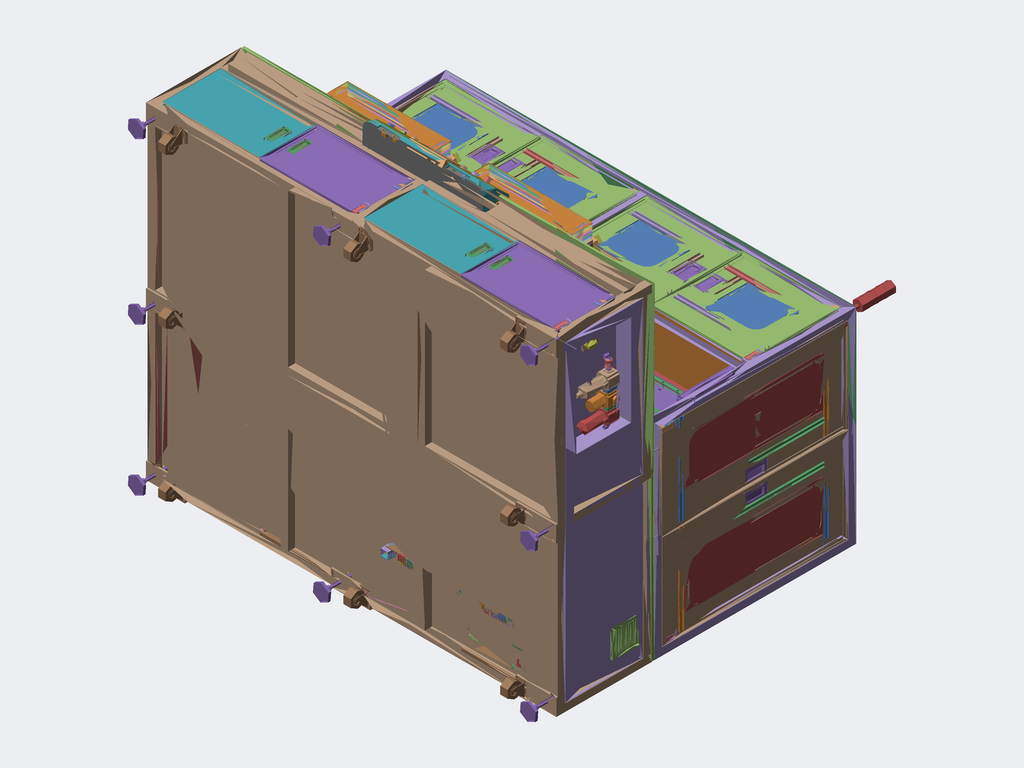Assembly | STEP file | 226 different items | 645 placed
Parts list (item | name | quantity | parent item | size | volume):
1 | ball screw nut-SFA3232-2.8 | x1 | - | 62 x 80 x 110 mm | 157675 mm3
2 | - | x1 | - | 31 x 2020 x 31 mm | 1487693 mm3
3 | HIWIN linear rail EGH30-1920-40-40 | x2 | in HIWIN linear rail EGH30CA | 28 x 23 x 1920 mm | 1071300 mm3
4 | HIWIN slider EGH30CA | x4 | in HIWIN linear rail EGH30CA | 60 x 32 x 99.1 mm | 151904 mm3
5 | - | x1 | - | 1970 x 20 x 225 mm | 8481911 mm3
6 | - | x1 | - | 11.5 x 66 x 40 mm | 3360 mm3
7 | - | x1 | - | 217 x 63 x 320 mm | 1789943 mm3
8 | - | x1 | - | 105 x 159 x 12 mm | 123349 mm3
9 | - | x1 | - | 319 x 74 x 2 mm | 46848 mm3
10 | - | x1 | - | 319 x 74 x 2 mm | 41628 mm3
11 | - | x1 | - | 100 x 108 x 18.001 mm | 56664 mm3
12 | - | x1 | - | 40 x 10 x 30 mm | 9955 mm3
13 | - | x1 | - | 110 x 160 x 60 mm | 79904 mm3
14 | - | x4 | - | 58 x 58 x 14 mm | 28098 mm3
15 | - | x1 | - | 152 x 125 x 238 mm | 147473 mm3
16 | - | x1 | - | 180 x 125 x 238 mm | 188317 mm3
17 | - | x2 | - | 230 x 2 x 105 mm | 25066 mm3
18 | - | x2 | - | - | -
19 | timing pulley C-HTPA30S5M250-A-N19 | x1 | - | 32 x 52 x 52 mm | 41096 mm3
20 | timing pulley C-HTPA30S5M250-A-N20 | x1 | - | 32 x 52 x 52 mm | 40136 mm3
21 | slot-type photoelectric sensor LU672-5N | x1 | - | 14.05 x 26.2 x 61.3 mm | 1669 mm3
22 | bearing fixing block BF25 | x1 | - | 30 x 106 x 80 mm | 180921 mm3
23 | bearing support block BK25 | x1 | - | 106 x 63 x 80 mm | 295057 mm3
24 | GB/T 894-2017 external retaining ring type A 25 | x1 | - | 27.3 x 30.557 x 1.2 mm | 213.948 mm3
25 | Heqi servo 1000W motor X2MA100A-N2L (aviation plug) | x1 | - | - | -
26 | - | x1 | - | 183.34 x 51.65 x 25 mm | 35272 mm3
27 | ball screw nut-SFS02525-1.8 | x2 | - | 48 x 62 x 60 mm | 60127 mm3
28 | - | x2 | - | 25 x 970 x 25 mm | 453168 mm3
29 | slider HGW30HC | x8 | - | 90 x 36 x 120.7 mm | 241575 mm3
30 | linear guide HGR30HC-1250-25-25 | x4 | - | 28 x 26 x 1250 mm | 722759 mm3
31 | - | x2 | in 211 | 570 x 570 x 15 mm | 4074607 mm3
32 | - | x2 | in 211 | 61.9 x 61.9 x 60 mm | 168821 mm3
33 | - | x4 | in 211 | 88 x 56 x 10 mm | 42549 mm3
34 | - | x2 | in 211 | 6.3 x 100 x 6.3 mm | 3083 mm3
35 | - | x2 | in 211 | 59.5 x 40 x 25 mm | 15043 mm3
36 | - | x4 | in 211 | 130 x 35 x 30 mm | 74604 mm3
37 | - | x4 | in 211 | 60 x 35 x 10 mm | 20336 mm3
38 | rotary cylinder ACKL32x90 | x4 | in 211 | 54 x 76 x 54 mm | 144312 mm3
39 | - | x2 | in 211 | 360 x 72.5 x 360 mm | 3129469 mm3
40 | - | x2 | in 211 | 419 x 78.97 x 419 mm | 4583187 mm3
41 | - | x2 | in 211 | 452 x 75.25 x 452 mm | 5130306 mm3
42 | - | x2 | in 211 | 520 x 79.32 x 520 mm | 7165293 mm3
43 | - | x4 | in Y-axis bellows cover assembly | 570 x 2 x 115 mm | 37091 mm3
44 | - | x4 | in Y-axis bellows cover assembly | 570 x 35 x 115.5 mm | 243087 mm3
45 | - | x4 | in Y-axis bellows cover assembly | - | -
46 | - | x2 | - | 80 x 85 x 125 mm | 372147 mm3
47 | - | x2 | - | 75 x 75 x 15 mm | 51651 mm3
48 | - | x2 | - | 65 x 82.5 x 45 mm | 171264 mm3
49 | - | x8 | - | 95 x 63 x 75 mm | 244424 mm3
50 | - | x2 | - | 13.5 x 37 x 40 mm | 2353 mm3
51 | - | x2 | - | 80 x 1.2 x 95 mm | 9034 mm3
52 | - | x4 | - | 35 x 20 x 30 mm | 2265 mm3
53 | - | x4 | - | 570 x 114 x 2 mm | 119896 mm3
54 | anti-collision silicone pad | x2 | - | 34 x 10 x 7 mm | 2064 mm3
55 | coupling DEP12-D40L-d17-e19-DC-DD | x2 | - | 66 x 40 x 41.384 mm | 61965 mm3
56 | GB/T 276-2013 deep groove ball bearing 6004-2RZ_6004-2RZ | x2 | - | 12 x 42 x 42 mm | 9713 mm3
57 | GB/T 894-2017[external retaining ring type A 20MM_20 | x2 | - | 22.1 x 25.046 x 1.2 mm | 154.505 mm3
58 | TBI bearing block FK20 | x2 | - | 85 x 85 x 64 mm | 139023 mm3
59 | Heqi 750W servo (SV-2MH075A-N2-LN wire type) | x2 | - | - | -
60 | slot-type photoelectric LU674-5NA | x2 | - | 15 x 16 x 28 mm | 2937 mm3
61 | - | x2 | - | 533 x 321 x 16 mm | 246500 mm3
62 | mirrored door latch (COMPANY_B) | x20 | in 68, 122, 127, 129 | 93 x 9.976 x 34.988 mm | 6427 mm3
63 | door latch (COMPANY_B) | x20 | in 68, 122, 127, 129 | 93 x 9.976 x 34.988 mm | 6427 mm3
64 | GY-AA29-AL06-96 nylon handle | x8 | in 68 | 43 x 107 x 15 mm | 16385 mm3
65 | door handle rear cover (SUS304) | x8 | in 68 | 47 x 108 x 11 mm | 7052 mm3
66 | - | x2 | in 68 | 533 x 321 x 15 mm | 244434 mm3
67 | - | x2 | - | 533 x 428 x 16 mm | 320755 mm3
68 | - | x2 | in 68 | 533 x 428 x 15 mm | 318433 mm3
69 | - | x1 | in 69 | 660.4 x 129.2 x 145.9 mm | 256487 mm3
70 | HMI touch panel SK-070QE.V1.5 | x1 | in 69 | 203 x 145 x 39 mm | 1003292 mm3
71 | three-pin two-speed power switch KCD4-16A-250 | x1 | in 69 | 21 x 15 x 27.336 mm | 4367 mm3
72 | illuminated flat push button white 24V | x1 | in 69 | 30 x 38 x 66.5 mm | 57717 mm3
73 | Yijia emergency stop switch | x1 | in 69 | 83 x 36 x 36 mm | 62929 mm3
74 | illuminated flat push button yellow 24V | x1 | in 69 | 30 x 38 x 66.5 mm | 57717 mm3
75 | illuminated flat push button green 24V | x2 | in 69 | 30 x 38 x 66.5 mm | 57717 mm3
76 | illuminated flat push button red 24V | x1 | in 69 | 30 x 38 x 66.5 mm | 57717 mm3
77 | USB interface | x2 | in 69 | 38 x 27 x 12 mm | 7027 mm3
78 | handheld controller connector DB9-RS232 | x1 | in 69 | 32 x 27 x 13 mm | 4868 mm3
79 | - | x1 | in 214 | 870 x 460 x 3 mm | 1176521 mm3
80 | power supply fixing sheet metal | x2 | in 214 | 15 x 20 x 10 mm | 522.847 mm3
81 | terminal stopper UK2.5B | x1 | in relay slot group | 43 x 36 x 10 mm | 8109 mm3
82 | terminal block UK2.5B | x30 | in relay slot group | 43 x 41 x 6 mm | 4189 mm3
83 | IDEC relay RJ1S-A220 | x3 | in relay slot group | 71 x 56 x 15 mm | 30075 mm3
84 | card slot 35-265 | x1 | in relay slot group | 35 x 6.5 x 265 mm | 13977 mm3
85 | - | x4 | in 214 | 40 x 38.5 x 480 mm | 109641 mm3
86 | Mean Well power supply LRS-350-24 | x1 | in 214 | - | -
87 | filter CW4EL2-30A-S | x1 | in 214 | 85 x 51 x 29 mm | 93702 mm3
88 | contactor NXC-12 | x1 | in 214 | 75 x 85 x 45 mm | 200816 mm3
89 | circuit breaker DZ267LE-32-10 | x1 | in 214 | 75.5 x 84 x 36 mm | 154947 mm3
90 | - | x3 | in 214 | 40 x 38.5 x 320 mm | 73088 mm3
91 | - | x1 | in 214 | 316 x 26 x 94 mm | 418687 mm3
92 | Puge 400W electric screwdriver driver | x3 | in 214 | - | -
93 | Heqi 750W servo driver (X3EA075A-A2) | x2 | in 214 | - | -
94 | Heqi 1000W servo driver SV-X3EA100A-A2 | x1 | in 214 | - | -
95 | - | x1 | in 168 | 2260 x 16 x 1812 mm | 64799622 mm3
96 | - | x1 | in 168 | 1718 x 428 x 15 mm | 1162465 mm3
97 | - | x1 | in 168 | 1718 x 428 x 87.5 mm | 1351126 mm3
98 | - | x1 | in 168 | 2260 x 525 x 1800 mm | 63757591 mm3
99 | - | x3 | in 168 | 30 x 67 x 20 mm | 5371 mm3
100 | - | x2 | in 168 | 38 x 142 x 10 mm | 51461 mm3
101 | - | x1 | in 168 | 71.5 x 31.5 x 125 mm | 22831 mm3
102 | silencer fixing block | x1 | in 168 | 60 x 25 x 20 mm | 24053 mm3
103 | large foot pad | x8 | in 168 | 96 x 166 x 96 mm | 161391 mm3
104 | universal caster-cf | x8 | in 168 | 115.75 x 105.5 x 64.5 mm | 273240 mm3
105 | power switch 2 | x1 | in 168 | 64.5 x 99 x 64.5 mm | 195044 mm3
106 | upright fitting KQ2H08-02AS | x2 | in 168 | 16.166 x 22 x 14 mm | 2374 mm3
107 | louvered fan grille LA751PBX0307 | x2 | in 168 | 151 x 151 x 33 mm | 559203 mm3
108 | 220V fan | x2 | in 168 | - | -
109 | hand slide valve HSV10 | x1 | in 110 | 35.5 x 35.5 x 68.5 mm | 34566 mm3
110 | pneumatic FRL unit GAC40010AS | x1 | in 110 | 248 x 227 x 99 mm | 1724530 mm3
111 | L-type fitting PL1003 | x2 | in 110 | 35.315 x 37 x 18 mm | 6710 mm3
112 | 1-branch plug | x2 | in four-station solenoid valve block-double head | 9.5 x 8 x 9.5 mm | 424.158 mm3
113 | 2-branch plug | x3 | in four-station solenoid valve block-double head | 13 x 9 x 13 mm | 992.021 mm3
114 | L-type fitting PL4-01 | x4 | in four-station solenoid valve block-double head | 22.874 x 22.3 x 11 mm | 1653 mm3
115 | L-type fitting PL6-01 | x1 | in four-station solenoid valve block-double head | 23.774 x 24.5 x 13 mm | 2165 mm3
116 | L-type fitting PL8-01 | x1 | in four-station solenoid valve block-double head | 29.374 x 27.1 x 15 mm | 3387 mm3
117 | single solenoid valve MVSD-180-4E1 | x2 | in four-station solenoid valve block-double head | 33.5 x 18 x 107 mm | 44857 mm3
118 | double solenoid valve 4V120-06 | x2 | in four-station solenoid valve block-double head | 33.5 x 18 x 144.5 mm | 59015 mm3
119 | - | x1 | in four-station solenoid valve block-double head | 95 x 25 x 58 mm | 76550 mm3
120 | upright fitting APC8-02 | x3 | in four-station solenoid valve block-double head | 25.7 x 16.166 x 15 mm | 2429 mm3
121 | - | x1 | in 168 | 2260 x 1110 x 1130 mm | 31144835 mm3
122 | - | x4 | in 122 | 523 x 1028 x 15 mm | 879625 mm3
123 | - | x4 | in 122 | 274 x 764 x 5 mm | 1044923 mm3
124 | door handle XAC81_A128 | x12 | in 122, 127, 129 | 128 x 19.001 x 83 mm | 21652 mm3
125 | magnetic latch HGE11-52-L150 | x12 | in 122, 127, 129 | 60 x 15 x 37 mm | 14160 mm3
126 | magnetic door catch | x8 | in 122, 127 | 53 x 13 x 25.5 mm | 11239 mm3
127 | - | x4 | in 127 | 533 x 1028 x 15 mm | 886970 mm3
128 | - | x4 | in 127 | 284 x 764 x 5 mm | 1083123 mm3
129 | - | x4 | in 129 | 533 x 508 x 15 mm | 546675 mm3
130 | - | x4 | in 129 | 284 x 244 x 5 mm | 344723 mm3
131 | - | x1 | in 168 | 1130 x 2260 x 2 mm | 5103955 mm3
132 | foldable alarm light | x1 | in 168 | 70 x 342 x 70 mm | 623933 mm3
133 | STD-NB1220 safety light curtain | x4 | in 168 | 29 x 296.5 x 27 mm | 192265 mm3
134 | LED 0.9M T8 tube, single-end input 30W ZKT8-9-A-12 | x2 | in 168 | - | -
135 | - | x1 | - | 1500 x 280 x 500 mm | 11121240 mm3
136 | - | x1 | - | 500 x 1500 x 10 mm | 7485180 mm3
137 | COMPANY_C blow-air scheme, large part | x1 | - | 475 x 570.585 x 525.846 mm | 39693153 mm3
138 | COMPANY_C blow-air scheme, small part | x2 | - | 330.519 x 479.611 x 400.249 mm | 15256287 mm3
139 | - | x3 | - | 45 x 20 x 13 mm | 10795 mm3
140 | - | x3 | - | 50 x 24 x 8 mm | 8483 mm3
141 | - | x1 | - | 12 x 37 x 18 mm | 4359 mm3
142 | - | x1 | - | 12 x 37 x 18 mm | 4359 mm3
143 | - | x6 | - | 8 x 23.5 x 5 mm | 825.463 mm3
144 | finger cylinder MHZL2-16D | x3 | - | 47 x 23.6 x 70 mm | 34913 mm3
145 | speed control fitting AS1201F-M5-04SA | x6 | - | 9.4 x 26.5 x 22 mm | 1970 mm3
146 | through-beam fiber sensor FT-D321Q-M | x6 | - | 3 x 3 x 21 mm | 128.837 mm3
147 | - | x2 | - | 17.3 x 24.5 x 17.3 mm | 2659 mm3
148 | - | x2 | - | 12 x 30 x 18 mm | 3302 mm3
149 | - | x2 | - | 12 x 30 x 18 mm | 3302 mm3
150 | - | x3 | - | 9.9 x 14.5 x 9.9 mm | 641.755 mm3
151 | - | x3 | - | 9.9 x 15.5 x 9.9 mm | 641.291 mm3
152 | - | x1 | - | 350 x 190 x 10 mm | 648871 mm3
153 | - | x1 | - | 180 x 12 x 70 mm | 130133 mm3
154 | - | x1 | - | 45 x 27.5 x 10 mm | 9795 mm3
155 | - | x1 | - | 30 x 40 x 18 mm | 14417 mm3
156 | - | x1 | - | 350 x 150 x 10 mm | 449712 mm3
157 | - | x6 | - | 20 x 20 x 110 mm | 33959 mm3
158 | - | x1 | - | 65 x 40 x 12 mm | 21976 mm3
159 | free-specified tolerance g6 equal-height bolt[HSBGFS6-30-5-5]_HSBGFS6-30-5-5 | x1 | - | 10 x 10 x 39 mm | 1235 mm3
160 | linear guide EGH15CA-360-30-30_L=360 | x2 | - | 15 x 300 x 12.5 mm | 45472 mm3
161 | linear rail slider EGH15CA | x8 | in lead screw 1.5Z module assembly-direct-400W_lead 10 | 34 x 19.5 x 57 mm | 29973 mm3
162 | pen-type cylinder MI16x200SCA | x1 | - | 311 x 25.403 x 22 mm | 38961 mm3
163 | fish-eye fitting F-M6X100U | x1 | - | - | 3624 mm3
164 | buffer ACJ1210 | x2 | - | 17 x 81.5 x 19.048 mm | 8306 mm3
165 | speed control fitting AS1201FM-M5E-06A | x2 | - | 10.4 x 26.5 x 23.3 mm | 2163 mm3
166 | - | x1 | in 214 | 170 x 70 x 20 mm | 204646 mm3
167 | - | x1 | in 214 | 150 x 95 x 12 mm | 149253 mm3
168 | - | x2 | in 214 | 25 x 72 x 25 mm | 22681 mm3
169 | - | x1 | in 214 | 25 x 65 x 25 mm | 11563 mm3
170 | - | x1 | in 214 | 166 x 12 x 40 mm | 14406 mm3
171 | - | x1 | in 214 | 40 x 45 x 40 mm | 6376 mm3
172 | - | x1 | in 214 | 61.928 x 48 x 180 mm | 40990 mm3
173 | drag chain fixing head FW175X40-XJT-W3D | x1 | in 214 | 39.75 x 19.5 x 48.2 mm | 4934 mm3
174 | material-separating mechanism drag chain | x1 | in 214 | 40 x 140 x 230 mm | 500295 mm3
175 | fiber amplifier FR-J16 | x3 | in 214 | - | -
176 | limit screw Y-JAB22-M6-L50 | x3 | in 214 | 60 x 15 x 15 mm | 3261 mm3
177 | - | x1 | in 32 | 170 x 1770 x 620 mm | 19562829 mm3
178 | - | x1 | in 32 | 1700 x 15 x 80 mm | 308828 mm3
179 | cable tray 40-60-490 | x2 | in 32 | 40 x 60 x 500 mm | 93421 mm3
180 | - | x1 | in 32 | 1732 x 250 x 75 mm | 5324161 mm3
181 | TBI ball screw 16-20-330 | x2 | - | 15 x 330 x 15 mm | 52902 mm3
182 | ball spline SFS01620-1.8 | x3 | - | 40 x 48 x 50 mm | 31024 mm3
183 | lead screw 1.5Z module-direct connection | x3 | in lead screw 1.5Z module assembly-direct-400W_lead 10 | 100 x 46 x 350 mm | 472702 mm3
184 | lead screw Z-axis upper cover plate-direct | x3 | in lead screw 1.5Z module assembly-direct-400W_lead 10 | 100 x 8 x 71 mm | 43189 mm3
185 | lead screw Z-axis lower cover plate | x3 | in lead screw 1.5Z module assembly-direct-400W_lead 10 | 100 x 8 x 71 mm | 53634 mm3
186 | lead screw fixing block - COMPANY_A version | x3 | in lead screw 1.5Z module assembly-direct-400W_lead 10 | 80 x 54.5 x 30 mm | 73786 mm3
187 | lead screw support block - COMPANY_A version | x3 | in lead screw 1.5Z module assembly-direct-400W_lead 10 | 80 x 54.5 x 14 mm | 35887 mm3
188 | lead screw 400W motor direct-connect flange | x3 | in lead screw 1.5Z module assembly-direct-400W_lead 10 | 60 x 30 x 60 mm | 61401 mm3
189 | X-axis lead screw slide - COMPANY_A version | x3 | in lead screw 1.5Z module assembly-direct-400W_lead 10 | 104 x 46 x 80 mm | 190847 mm3
190 | 1.5Z axis cover plate_3X cover plate | x3 | in lead screw 1.5Z module assembly-direct-400W_lead 10 | 79 x 6 x 366 mm | 77305 mm3
191 | lead screw origin sensing plate | x3 | in lead screw 1.5Z module assembly-direct-400W_lead 10 | 43 x 9 x 10 mm | 314.784 mm3
192 | bearing cover plate | x3 | in lead screw 1.5Z module assembly-direct-400W_lead 10 | 38 x 38 x 2 mm | 1706 mm3
193 | steel sleeve 12-14-10 | x3 | in lead screw 1.5Z module assembly-direct-400W_lead 10 | 14 x 14 x 10 mm | 408.407 mm3
194 | small slot-type switch DC-SPX205 | x3 | in lead screw 1.5Z module assembly-direct-400W_lead 10 | 20.5 x 12 x 13.4 mm | 1038 mm3
195 | - | x3 | in lead screw 1.5Z module assembly-direct-400W_lead 10 | 10.153 x 20.245 x 20.375 mm | 1688 mm3
196 | linear guide EGH15CA-240-30-30_L=560 | x6 | in lead screw 1.5Z module assembly-direct-400W_lead 10 | 15 x 240 x 12.5 mm | 36704 mm3
197 | ball bearing-B6000ZZ | x3 | in lead screw 1.5Z module assembly-direct-400W_lead 10 | 8 x 26 x 26 mm | 2612 mm3
198 | ball bearing_B6001.5ZZ | x6 | in lead screw 1.5Z module assembly-direct-400W_lead 10 | 8 x 28 x 28 mm | 3774 mm3
199 | bumper sleeve 12-M4 | x12 | in lead screw 1.5Z module assembly-direct-400W_lead 10 | 12 x 10 x 12 mm | 1005 mm3
200 | coupling GHBG   LF-D-30-10-14 | x3 | in lead screw 1.5Z module assembly-direct-400W_lead 10 | 30 x 30 x 37 mm | 19540 mm3
201 | Heqi servo 400W X2MA040A-B (wire type) | x3 | in lead screw 1.5Z module assembly-direct-400W_lead 10 | - | -
202 | TBI ball screw 16-10-330 | x1 | - | 15 x 330 x 15 mm | 52902 mm3
203 | PN_0001-1.5Z direct-connect drag chain fixing piece | x1 | in lead screw 1.5Z module assembly-direct-400W_lead 10 | 170 x 185 x 51 mm | 121882 mm3
204 | - | x3 | - | 95 x 60 x 20 mm | 58909 mm3
205 | - | x6 | - | 8 x 8 x 65 mm | 2978 mm3
206 | linear bearing LMH8UU | x6 | - | 24 x 32 x 21 mm | 5040 mm3
207 | spring 2 | x6 | - | 9.6 x 9.6 x 35 mm | 344.84 mm3
208 | - | x3 | - | 105 x 12 x 290 mm | 325340 mm3
209 | - | x3 | - | 95 x 10 x 70 mm | 48778 mm3
210 | - | x3 | - | 40 x 25 x 53 mm | 43545 mm3
211 | - | x2 | - | 14 x 90 x 14 mm | 10470 mm3
212 | - | x1 | - | 6 x 126 x 6 mm | 3480 mm3
213 | - | x3 | - | 90 x 113 x 20 mm | 17947 mm3
214 | - | x3 | - | 12 x 49.5 x 12 mm | 5016 mm3
215 | coupling DCQ03-D32-d12-e14 | x3 | - | 32 x 32 x 31.992 mm | 20201 mm3
216 | ball bearing_B6001ZZ | x3 | - | 8 x 28 x 28 mm | 3774 mm3
217 | KTC linear displacement sensor KTC2-50MM | x3 | in KTC linear displacement sensor KTC-50MM assembly | 36 x 33.3 x 269 mm | 80429 mm3
218 | KTC displacement sensor fixing sheet metal | x6 | in KTC linear displacement sensor KTC-50MM assembly | 42 x 9 x 9 mm | 488.862 mm3
219 | Heqi 400W motor X2MH040A-N2L (wire type) | x3 | - | 60 x 76.95 x 117.5 mm | 299796 mm3
220 | hex socket M4x0 | x3 | - | 7 x 9 x 7 mm | 199.204 mm3
221 | hex socket M5x12 | x6 | in hex socket M5x12+M5 flat washer+M5 spring washer | 8.5 x 17 x 8.5 mm | 481.648 mm3
222 | M5 spring washer | x6 | in hex socket M5x12+M5 flat washer+M5 spring washer | 9.15 x 1.2 x 9.15 mm | 52.779 mm3
223 | M5 flat washer | x6 | in hex socket M5x12+M5 flat washer+M5 spring washer | 10 x 1 x 10 mm | 56.478 mm3
224 | - | x1 | - | 6 x 126 x 6 mm | 3530 mm3
225 | - | x1 | - | 20 x 59 x 20 mm | 11876 mm3
226 | - | x1 | - | 14 x 99 x 14 mm | 5187 mm3
Placements (level | parent | child | x y z in mm | rotation matrix by rows), first 333 of 718 lines:
1 | LB1581SSX3315 | subassembly 2 | -10.0 1154.0 -175.0 | 1 0 0 0 1 0 0 0 1
2 | subassembly 2 | subassembly 3 | 401.538 223.266 107.894 | 0 0 -1 1 0 0 0 -1 -0
3 | subassembly 3 | ball screw nut-SFA3232-2.8 | -223.266 46.894 1318.538 | 0 -1 0 -1 0 0 0 0 -1
3 | subassembly 3 | subassembly 4 | -223.266 46.894 1437.538 | 0 0 1 -1 0 0 0 -1 -0
2 | subassembly 2 | HIWIN linear rail EGH30CA | -890.0 -54.361 26.062 | 0 0 -1 -1 0 0 0 1 0
3 | HIWIN linear rail EGH30CA | HIWIN linear rail EGH30-1920-40-40 | 21.639 14.938 -0.0 | 1 0 0 0 1 0 0 0 1
3 | HIWIN linear rail EGH30CA | HIWIN slider EGH30CA | 21.639 14.938 -4.95 | 1 0 0 0 1 0 0 0 1
3 | HIWIN linear rail EGH30CA | HIWIN slider EGH30CA | 21.639 14.938 -214.95 | 1 0 0 0 1 0 0 0 1
2 | subassembly 2 | HIWIN linear rail EGH30CA | -890.0 97.639 26.062 | 0 0 -1 -1 0 0 0 1 0
3 | HIWIN linear rail EGH30CA | HIWIN linear rail EGH30-1920-40-40 | 21.639 14.938 0.0 | 1 0 0 0 1 0 0 0 1
3 | HIWIN linear rail EGH30CA | HIWIN slider EGH30CA | 21.639 14.938 -4.95 | 1 0 0 0 1 0 0 0 1
3 | HIWIN linear rail EGH30CA | HIWIN slider EGH30CA | 21.639 14.938 -214.95 | 1 0 0 0 1 0 0 0 1
2 | subassembly 2 | subassembly 5 | 0.0 -0.0 20.0 | -1 0 0 0 0 -1 0 -1 0
2 | subassembly 2 | subassembly 6 | -700.0 -110.5 63.132 | 0 0 -1 -1 0 0 0 1 -0
2 | subassembly 2 | subassembly 7 | -905.0 -0.0 57.0 | 0 0 -1 -1 0 0 0 1 -0
2 | subassembly 2 | subassembly 8 | -985.0 -0.0 -9.0 | 0 0 -1 -1 0 0 0 1 -0
2 | subassembly 2 | subassembly 9 | -745.0 110.5 59.0 | -1 0 0 0 0 1 0 1 0
2 | subassembly 2 | subassembly 10 | -745.0 -110.5 59.0 | 1 0 0 0 0 -1 0 1 0
2 | subassembly 2 | subassembly 11 | -1005.0 0.0 -70.69 | 0 0 -1 -1 0 0 0 1 -0
2 | subassembly 2 | subassembly 12 | -1000.0 -0.0 -139.0 | 0 0 1 -1 0 0 0 -1 0
2 | subassembly 2 | subassembly 12 | -1045.0 -0.0 -62.0 | 0 0 -1 -1 0 0 0 1 -0
2 | subassembly 2 | subassembly 13 | -943.75 0.0 61.0 | 0 0 1 -0.9905 0.1372 0 -0.1372 -0.9905 0
2 | subassembly 2 | subassembly 13 | 940.0 0.0 61.0 | 0 0 1 -0.994 0.109 0 -0.109 -0.994 0
2 | subassembly 2 | subassembly 14 | -987.0 -0.0 18.0 | 1 0 0 0 0 -1 0 1 -0
2 | subassembly 2 | subassembly 15 | 987.0 0.0 18.0 | -1 0 0 0 0 1 0 1 0
2 | subassembly 2 | subassembly 16 | -905.0 0.0 73.5 | 0 1 0 1 0 0 0 0 -1
2 | subassembly 2 | subassembly 16 | -585.0 0.0 73.5 | 0 -1 0 -1 0 0 0 0 -1
2 | subassembly 2 | subassembly 17 | -1072.9 -115.0 21.0 | 1 0 0 0 1 0 0 0 1
2 | subassembly 2 | subassembly 17 | -417.1 115.0 21.0 | -1 0 0 0 -1 0 0 0 1
2 | subassembly 2 | timing pulley C-HTPA30S5M250-A-N19 | -1038.0 -0.0 -70.69 | 1 0 0 0 0.3847 -0.923 0 0.923 0.3847
2 | subassembly 2 | timing pulley C-HTPA30S5M250-A-N20 | -1038.0 0.0 61.0 | 1 0 0 0 0.7853 0.6191 0 -0.6191 0.7853
2 | subassembly 2 | slot-type photoelectric sensor LU672-5N | -732.854 -123.352 -43.15 | 0 1 0 -1 0 0 0 0 1
2 | subassembly 2 | bearing fixing block BF25 | 939.0 0.0 13.0 | 1 0 0 0 -1 0 0 0 -1
2 | subassembly 2 | bearing support block BK25 | -829.555 -0.0 -38.895 | 0 1 0 -1 0 0 0 0 1
2 | subassembly 2 | GB/T 894-2017 external retaining ring type A 25 | 979.6 0.0 61.0 | 0 0 1 0.6431 0.7658 0 -0.7658 0.6431 0
2 | subassembly 2 | Heqi servo 1000W motor X2MA100A-N2L (aviation plug) | -985.0 -0.0 39.31 | 0 0 -1 -1 0 0 0 1 0
2 | subassembly 2 | subassembly 18 | -1035.5 21.313 52.775 | 0 0 -1 0 1 0 1 0 0
1 | LB1581SSX3315 | subassembly 19 | 390.0 646.5 -325.0 | 0 1 0 0 0 1 1 0 -0
2 | subassembly 19 | subassembly 20 | 1362.538 223.266 89.394 | 0 0 -1 1 0 0 0 -1 0
3 | subassembly 20 | ball screw nut-SFS02525-1.8 | -223.266 46.894 550.538 | 0 -1 0 -1 0 0 0 0 -1
3 | subassembly 20 | subassembly 21 | -223.266 46.894 1437.538 | 0 0 1 -1 0 0 0 -1 -0
2 | subassembly 19 | subassembly 22 | -74.808 -214.878 5.532 | 0 0 -1 -1 0 0 0 1 0
3 | subassembly 22 | slider HGW30HC | 0.1218 20.468 -771.308 | 1 0 0 0 1 0 0 0 1
3 | subassembly 22 | linear guide HGR30HC-1250-25-25 | 0.1218 20.468 0.1918 | 1 0 0 0 1 0 0 0 1
3 | subassembly 22 | slider HGW30HC | 0.1218 20.468 -1071.308 | 1 0 0 0 1 0 0 0 1
2 | subassembly 19 | subassembly 22 | -74.808 215.122 5.532 | 0 0 -1 -1 0 0 0 1 0
3 | subassembly 22 | slider HGW30HC | 0.1218 20.468 -771.308 | 1 0 0 0 1 0 0 0 1
3 | subassembly 22 | linear guide HGR30HC-1250-25-25 | 0.1218 20.468 0.1918 | 1 0 0 0 1 0 0 0 1
3 | subassembly 22 | slider HGW30HC | 0.1218 20.468 -1071.308 | 1 0 0 0 1 0 0 0 1
2 | subassembly 19 | subassembly 23 | 862.511 7.035 108.0 | 0 -1 0 1 0 0 0 0 1
3 | subassembly 23 | subassembly 24 | -7.035 16.011 -0.0 | 1 0 0 0 1 0 0 0 1
3 | subassembly 23 | subassembly 13 | -7.035 16.011 37.5 | 1 0 0 0 1 0 0 0 1
3 | subassembly 23 | subassembly 25 | 202.571 -193.596 12.5 | 0.7071 -0.7071 0 0.7071 0.7071 0 0 0 1
3 | subassembly 23 | subassembly 25 | -221.111 230.087 12.5 | 0.7071 -0.7071 0 0.7071 0.7071 0 0 0 1
3 | subassembly 23 | subassembly 26 | 47.62 -134.152 -15.5 | 0.2658 0 0.964 0.964 0 -0.2658 0 1 0
3 | subassembly 23 | subassembly 26 | 52.75 -148.248 4.0 | 0.9397 -0.342 0 0.342 0.9397 0 0 0 1
3 | subassembly 23 | subassembly 23 | -183.634 192.61 95.968 | -0.7071 -0.7071 0 0.7071 -0.7071 0 0 0 1
3 | subassembly 23 | subassembly 23 | 165.095 -156.119 101.82 | 0.7071 0.7071 0 -0.7071 0.7071 0 0 0 1
3 | subassembly 23 | subassembly 27 | -158.886 167.861 75.968 | 0.7071 0.7071 0 -0.7071 0.7071 0 0 0 1
3 | subassembly 23 | subassembly 27 | 140.346 -131.37 81.82 | -0.7071 0.7071 0 0.7071 0.7071 0 0 0 -1
3 | subassembly 23 | rotary cylinder ACKL32x90 | 202.571 -193.596 17.5 | 0.7071 0 0.7071 0.7071 0 -0.7071 0 1 -0
3 | subassembly 23 | rotary cylinder ACKL32x90 | -221.111 230.087 17.5 | 0.7071 0 0.7071 0.7071 0 -0.7071 0 1 -0
3 | subassembly 23 | subassembly 28 | -7.035 16.011 7.5 | -0.4848 0 -0.8746 -0.8746 0 0.4848 0 1 0
3 | subassembly 23 | subassembly 29 | -7.035 16.011 7.5 | -0.4848 0 -0.8746 -0.8746 0 0.4848 0 1 0
3 | subassembly 23 | subassembly 30 | -7.035 16.011 7.5 | -0.4848 0 -0.8746 -0.8746 0 0.4848 0 1 0
3 | subassembly 23 | subassembly 31 | -7.035 16.011 7.5 | -0.4848 0 -0.8746 -0.8746 0 0.4848 0 1 0
2 | subassembly 19 | Y-axis bellows cover assembly | -955.939 -33.475 113.73 | 1 0 0 0 1 0 0 0 1
3 | Y-axis bellows cover assembly | subassembly 32 | 749.439 33.475 -55.73 | 0 1 0 1 0 0 0 0 -1
3 | Y-axis bellows cover assembly | subassembly 33 | 654.439 33.475 -55.98 | 0 -1 0 -1 0 0 0 0 -1
3 | Y-axis bellows cover assembly | subassembly 34 | 657.539 -251.525 -113.23 | 1 0 0 0 1 0 0 0 1
2 | subassembly 19 | Y-axis bellows cover assembly | 1880.939 33.475 113.73 | -1 0 0 0 -1 0 0 0 1
3 | Y-axis bellows cover assembly | subassembly 32 | 749.439 33.475 -55.73 | 0 1 0 1 0 0 0 0 -1
3 | Y-axis bellows cover assembly | subassembly 33 | 654.439 33.475 -55.98 | 0 -1 0 -1 0 0 0 0 -1
3 | Y-axis bellows cover assembly | subassembly 34 | 657.539 -251.525 -113.23 | 1 0 0 0 1 0 0 0 1
2 | subassembly 19 | subassembly 35 | -0.0 0.0 42.5 | 0 0 -1 -1 0 0 0 1 0
2 | subassembly 19 | subassembly 36 | 893.5 -0.0 37.5 | 0 0 -1 1 0 0 0 -1 0
2 | subassembly 19 | subassembly 37 | 846.5 0.0 19.5 | 0 0 -1 -1 0 0 0 1 0
2 | subassembly 19 | subassembly 38 | 696.5 -215.0 42.0 | 0 0 -1 -1 0 0 0 1 -0
2 | subassembly 19 | subassembly 38 | 996.5 -215.0 42.0 | 0 0 -1 -1 0 0 0 1 -0
2 | subassembly 19 | subassembly 38 | 996.5 215.0 42.0 | 0 0 -1 -1 0 0 0 1 0
2 | subassembly 19 | subassembly 38 | 696.5 215.0 42.0 | 0 0 -1 -1 0 0 0 1 0
2 | subassembly 19 | subassembly 39 | 866.5 -34.5 27.0 | 0 0 -1 -1 0 0 0 1 0
2 | subassembly 19 | subassembly 40 | -77.5 0.0 83.0 | 0 0 -1 1 0 0 0 -1 -0
2 | subassembly 19 | subassembly 41 | 1101.5 285.0 120.5 | 0 0 1 1 0 0 0 1 -0
2 | subassembly 19 | subassembly 41 | 1101.5 -285.0 120.5 | 0 0 -1 -1 0 0 0 1 0
2 | subassembly 19 | subassembly 12 | 846.5 285.0 58.5 | 1 0 0 0 0 -1 0 1 0
2 | subassembly 19 | subassembly 12 | 846.5 -287.0 58.5 | 1 0 0 0 0 -1 0 1 0
2 | subassembly 19 | subassembly 13 | 22.0 0.0 42.5 | 0 0 1 0.9958 -0.09115 0 0.09115 0.9958 -0
2 | subassembly 19 | anti-collision silicone pad | 869.0 0.0 80.0 | 0 0 1 1 0 0 0 1 -0
2 | subassembly 19 | coupling DEP12-D40L-d17-e19-DC-DD | -49.0 0.0 42.5 | 1 0 0 0 -0.8692 0.4944 0 -0.4944 -0.8692
2 | subassembly 19 | GB/T 276-2013 deep groove ball bearing 6004-2RZ_6004-2RZ | 885.5 0.0 42.5 | -1 0 0 0 -0.03697 0.9993 0 0.9993 0.03697
2 | subassembly 19 | GB/T 894-2017[external retaining ring type A 20MM_20 | 892.1 0.0 42.5 | 0 0 -1 1 -0.003491 0 -0.003491 -1 0
2 | subassembly 19 | TBI bearing block FK20 | 12.0 69.837 105.244 | 0 0 -1 -0.7071 0.7071 0 0.7071 0.7071 0
2 | subassembly 19 | Heqi 750W servo (SV-2MH075A-N2-LN wire type) | -122.0 0.0 42.5 | 0 0 1 0.01657 -0.9999 0 0.9999 0.01657 -0
2 | subassembly 19 | slot-type photoelectric LU674-5NA | 855.5 -45.0 -0.0 | 0 0 -1 -1 0 0 0 1 -0
1 | LB1581SSX3315 | subassembly 19 | -390.0 646.5 -325.0 | 0 1 0 0 0 1 1 0 -0
2 | subassembly 19 | subassembly 20 | 1362.538 223.266 89.394 | 0 0 -1 1 0 0 0 -1 0
3 | subassembly 20 | ball screw nut-SFS02525-1.8 | -223.266 46.894 550.538 | 0 -1 0 -1 0 0 0 0 -1
3 | subassembly 20 | subassembly 21 | -223.266 46.894 1437.538 | 0 0 1 -1 0 0 0 -1 -0
2 | subassembly 19 | subassembly 22 | -74.808 -214.878 5.532 | 0 0 -1 -1 0 0 0 1 0
3 | subassembly 22 | slider HGW30HC | 0.1218 20.468 -771.308 | 1 0 0 0 1 0 0 0 1
3 | subassembly 22 | linear guide HGR30HC-1250-25-25 | 0.1218 20.468 0.1918 | 1 0 0 0 1 0 0 0 1
3 | subassembly 22 | slider HGW30HC | 0.1218 20.468 -1071.308 | 1 0 0 0 1 0 0 0 1
2 | subassembly 19 | subassembly 22 | -74.808 215.122 5.532 | 0 0 -1 -1 0 0 0 1 0
3 | subassembly 22 | slider HGW30HC | 0.1218 20.468 -771.308 | 1 0 0 0 1 0 0 0 1
3 | subassembly 22 | linear guide HGR30HC-1250-25-25 | 0.1218 20.468 0.1918 | 1 0 0 0 1 0 0 0 1
3 | subassembly 22 | slider HGW30HC | 0.1218 20.468 -1071.308 | 1 0 0 0 1 0 0 0 1
2 | subassembly 19 | subassembly 23 | 862.511 7.035 108.0 | 0 -1 0 1 0 0 0 0 1
3 | subassembly 23 | subassembly 24 | -7.035 16.011 -0.0 | 1 0 0 0 1 0 0 0 1
3 | subassembly 23 | subassembly 13 | -7.035 16.011 37.5 | 1 0 0 0 1 0 0 0 1
3 | subassembly 23 | subassembly 25 | 202.571 -193.596 12.5 | 0.7071 -0.7071 0 0.7071 0.7071 0 0 0 1
3 | subassembly 23 | subassembly 25 | -221.111 230.087 12.5 | 0.7071 -0.7071 0 0.7071 0.7071 0 0 0 1
3 | subassembly 23 | subassembly 26 | 47.62 -134.152 -15.5 | 0.2658 0 0.964 0.964 0 -0.2658 0 1 0
3 | subassembly 23 | subassembly 26 | 52.75 -148.248 4.0 | 0.9397 -0.342 0 0.342 0.9397 0 0 0 1
3 | subassembly 23 | subassembly 23 | -183.634 192.61 95.968 | -0.7071 -0.7071 0 0.7071 -0.7071 0 0 0 1
3 | subassembly 23 | subassembly 23 | 165.095 -156.119 101.82 | 0.7071 0.7071 0 -0.7071 0.7071 0 0 0 1
3 | subassembly 23 | subassembly 27 | -158.886 167.861 75.968 | 0.7071 0.7071 0 -0.7071 0.7071 0 0 0 1
3 | subassembly 23 | subassembly 27 | 140.346 -131.37 81.82 | -0.7071 0.7071 0 0.7071 0.7071 0 0 0 -1
3 | subassembly 23 | rotary cylinder ACKL32x90 | 202.571 -193.596 17.5 | 0.7071 0 0.7071 0.7071 0 -0.7071 0 1 -0
3 | subassembly 23 | rotary cylinder ACKL32x90 | -221.111 230.087 17.5 | 0.7071 0 0.7071 0.7071 0 -0.7071 0 1 -0
3 | subassembly 23 | subassembly 28 | -7.035 16.011 7.5 | -0.4848 0 -0.8746 -0.8746 0 0.4848 0 1 0
3 | subassembly 23 | subassembly 29 | -7.035 16.011 7.5 | -0.4848 0 -0.8746 -0.8746 0 0.4848 0 1 0
3 | subassembly 23 | subassembly 30 | -7.035 16.011 7.5 | -0.4848 0 -0.8746 -0.8746 0 0.4848 0 1 0
3 | subassembly 23 | subassembly 31 | -7.035 16.011 7.5 | -0.4848 0 -0.8746 -0.8746 0 0.4848 0 1 0
2 | subassembly 19 | Y-axis bellows cover assembly | -955.939 -33.475 113.73 | 1 0 0 0 1 0 0 0 1
3 | Y-axis bellows cover assembly | subassembly 32 | 749.439 33.475 -55.73 | 0 1 0 1 0 0 0 0 -1
3 | Y-axis bellows cover assembly | subassembly 33 | 654.439 33.475 -55.98 | 0 -1 0 -1 0 0 0 0 -1
3 | Y-axis bellows cover assembly | subassembly 34 | 657.539 -251.525 -113.23 | 1 0 0 0 1 0 0 0 1
2 | subassembly 19 | Y-axis bellows cover assembly | 1880.939 33.475 113.73 | -1 0 0 0 -1 0 0 0 1
3 | Y-axis bellows cover assembly | subassembly 32 | 749.439 33.475 -55.73 | 0 1 0 1 0 0 0 0 -1
3 | Y-axis bellows cover assembly | subassembly 33 | 654.439 33.475 -55.98 | 0 -1 0 -1 0 0 0 0 -1
3 | Y-axis bellows cover assembly | subassembly 34 | 657.539 -251.525 -113.23 | 1 0 0 0 1 0 0 0 1
2 | subassembly 19 | subassembly 35 | 0.0 0.0 42.5 | 0 0 -1 -1 0 0 0 1 -0
2 | subassembly 19 | subassembly 36 | 893.5 -0.0 37.5 | 0 0 -1 1 0 0 0 -1 0
2 | subassembly 19 | subassembly 37 | 846.5 0.0 19.5 | 0 0 -1 -1 0 0 0 1 0
2 | subassembly 19 | subassembly 38 | 696.5 -215.0 42.0 | 0 0 -1 -1 0 0 0 1 -0
2 | subassembly 19 | subassembly 38 | 996.5 -215.0 42.0 | 0 0 -1 -1 0 0 0 1 -0
2 | subassembly 19 | subassembly 38 | 996.5 215.0 42.0 | 0 0 -1 -1 0 0 0 1 -0
2 | subassembly 19 | subassembly 38 | 696.5 215.0 42.0 | 0 0 -1 -1 0 0 0 1 -0
2 | subassembly 19 | subassembly 39 | 866.5 -34.5 27.0 | 0 0 -1 -1 0 0 0 1 0
2 | subassembly 19 | subassembly 40 | -77.5 0.0 83.0 | 0 0 -1 1 0 0 0 -1 -0
2 | subassembly 19 | subassembly 41 | 1101.5 285.0 120.5 | 0 0 1 1 0 0 0 1 -0
2 | subassembly 19 | subassembly 41 | 1101.5 -285.0 120.5 | 0 0 -1 -1 0 0 0 1 0
2 | subassembly 19 | subassembly 12 | 846.5 285.0 58.5 | 1 0 0 0 0 -1 0 1 0
2 | subassembly 19 | subassembly 12 | 846.5 -287.0 58.5 | 1 0 0 0 0 -1 0 1 0
2 | subassembly 19 | subassembly 13 | 22.0 0.0 42.5 | 0 0 1 0.9958 -0.09115 0 0.09115 0.9958 -0
2 | subassembly 19 | anti-collision silicone pad | 869.0 0.0 80.0 | 0 0 1 1 0 0 0 1 -0
2 | subassembly 19 | coupling DEP12-D40L-d17-e19-DC-DD | -49.0 0.0 42.5 | 1 0 0 0 -0.8692 0.4944 0 -0.4944 -0.8692
2 | subassembly 19 | GB/T 276-2013 deep groove ball bearing 6004-2RZ_6004-2RZ | 885.5 0.0 42.5 | -1 0 0 0 -0.03697 0.9993 0 0.9993 0.03697
2 | subassembly 19 | GB/T 894-2017[external retaining ring type A 20MM_20 | 892.1 0.0 42.5 | 0 0 -1 1 -0.003491 0 -0.003491 -1 0
2 | subassembly 19 | TBI bearing block FK20 | 12.0 69.837 105.244 | 0 0 -1 -0.7071 0.7071 0 0.7071 0.7071 0
2 | subassembly 19 | Heqi 750W servo (SV-2MH075A-N2-LN wire type) | -122.0 0.0 42.5 | 0 0 1 0.01657 -0.9999 0 0.9999 0.01657 -0
2 | subassembly 19 | slot-type photoelectric LU674-5NA | 855.5 -45.0 -0.0 | 0 0 -1 -1 0 0 0 1 -0
1 | LB1581SSX3315 | subassembly 18 | -1130.0 646.5 900.0 | 1 0 0 0 0 -1 0 1 0
2 | subassembly 18 | subassembly 42 | 41.0 0.0 329.5 | 1 0 0 0 0 1 0 -1 0
3 | subassembly 42 | subassembly 43 | 266.5 -0.0 -0.0 | -1 0 0 0 -1 0 0 0 1
3 | subassembly 42 | mirrored door latch (COMPANY_B) | 84.258 -146.492 29.428 | 0 0 1 -1 0 0 0 -1 -0
3 | subassembly 42 | door latch (COMPANY_B) | 84.258 146.492 29.428 | 0 0 -1 1 0 0 0 -1 0
3 | subassembly 42 | GY-AA29-AL06-96 nylon handle | 474.5 53.5 -11.0 | 1 0 0 0 -1 0 0 0 -1
3 | subassembly 42 | door handle rear cover (SUS304) | 469.746 42.417 -11.2 | 1 0 0 0 1 0 0 0 1
2 | subassembly 18 | subassembly 44 | 842.5 0.0 329.5 | 1 0 0 0 0 1 0 -1 0
3 | subassembly 44 | subassembly 44 | 0.0 0.0 -0.0 | 1 0 0 0 1 0 0 0 1
3 | subassembly 44 | mirrored door latch (COMPANY_B) | 182.242 146.492 29.428 | 0 0 -1 1 0 0 0 -1 0
3 | subassembly 44 | door latch (COMPANY_B) | 182.242 -146.492 29.428 | 0 0 1 -1 0 0 0 -1 0
3 | subassembly 44 | door handle rear cover (SUS304) | -212.754 42.417 -11.2 | 1 0 0 0 1 0 0 0 1
3 | subassembly 44 | GY-AA29-AL06-96 nylon handle | -208.0 53.5 -11.0 | 1 0 0 0 -1 0 0 0 -1
2 | subassembly 18 | subassembly 44 | 1952.5 -0.0 329.5 | 1 0 0 0 0 1 0 -1 0
3 | subassembly 44 | subassembly 44 | 0.0 0.0 -0.0 | 1 0 0 0 1 0 0 0 1
3 | subassembly 44 | mirrored door latch (COMPANY_B) | 182.242 146.492 29.428 | 0 0 -1 1 0 0 0 -1 0
3 | subassembly 44 | door latch (COMPANY_B) | 182.242 -146.492 29.428 | 0 0 1 -1 0 0 0 -1 0
3 | subassembly 44 | door handle rear cover (SUS304) | -212.754 42.417 -11.2 | 1 0 0 0 1 0 0 0 1
3 | subassembly 44 | GY-AA29-AL06-96 nylon handle | -208.0 53.5 -11.0 | 1 0 0 0 -1 0 0 0 -1
2 | subassembly 18 | subassembly 42 | 1151.0 -0.0 329.5 | 1 0 0 0 0 1 0 -1 0
3 | subassembly 42 | subassembly 43 | 266.5 -0.0 -0.0 | -1 0 0 0 -1 0 0 0 1
3 | subassembly 42 | mirrored door latch (COMPANY_B) | 84.258 -146.492 29.428 | 0 0 1 -1 0 0 0 -1 -0
3 | subassembly 42 | door latch (COMPANY_B) | 84.258 146.492 29.428 | 0 0 -1 1 0 0 0 -1 0
3 | subassembly 42 | GY-AA29-AL06-96 nylon handle | 474.5 53.5 -11.0 | 1 0 0 0 -1 0 0 0 -1
3 | subassembly 42 | door handle rear cover (SUS304) | 469.746 42.417 -11.2 | 1 0 0 0 1 0 0 0 1
2 | subassembly 18 | subassembly 42 | 2219.0 -1798.0 276.0 | -1 0 0 0 0 -1 0 -1 0
3 | subassembly 42 | subassembly 43 | 266.5 -0.0 -0.0 | -1 0 0 0 -1 0 0 0 1
3 | subassembly 42 | GY-AA29-AL06-96 nylon handle | 474.5 53.5 -11.0 | 1 0 0 0 -1 0 0 0 -1
3 | subassembly 42 | door handle rear cover (SUS304) | 469.746 42.417 -11.2 | 1 0 0 0 1 0 0 0 1
3 | subassembly 42 | mirrored door latch (COMPANY_B) | 84.258 -199.992 29.428 | 0 0 1 -1 0 0 0 -1 -0
3 | subassembly 42 | door latch (COMPANY_B) | 84.258 199.992 29.428 | 0 0 -1 1 0 0 0 -1 0
2 | subassembly 18 | subassembly 44 | 1417.5 -1798.0 276.0 | -1 0 0 0 0 -1 0 -1 0
3 | subassembly 44 | subassembly 44 | -0.0 0.0 -0.0 | 1 0 0 0 1 0 0 0 1
3 | subassembly 44 | mirrored door latch (COMPANY_B) | 182.242 199.992 29.428 | 0 0 -1 1 0 0 0 -1 0
3 | subassembly 44 | door latch (COMPANY_B) | 182.242 -199.992 29.428 | 0 0 1 -1 0 0 0 -1 0
3 | subassembly 44 | GY-AA29-AL06-96 nylon handle | -208.0 53.5 -11.0 | 1 0 0 0 -1 0 0 0 -1
3 | subassembly 44 | door handle rear cover (SUS304) | -212.754 42.417 -11.2 | 1 0 0 0 1 0 0 0 1
2 | subassembly 18 | subassembly 44 | 307.5 -1800.0 276.0 | -1 0 0 0 0 -1 0 -1 0
3 | subassembly 44 | subassembly 44 | -0.0 0.0 -0.0 | 1 0 0 0 1 0 0 0 1
3 | subassembly 44 | mirrored door latch (COMPANY_B) | 182.242 199.992 29.428 | 0 0 -1 1 0 0 0 -1 0
3 | subassembly 44 | door latch (COMPANY_B) | 182.242 -199.992 29.428 | 0 0 1 -1 0 0 0 -1 0
3 | subassembly 44 | GY-AA29-AL06-96 nylon handle | -208.0 53.5 -11.0 | 1 0 0 0 -1 0 0 0 -1
3 | subassembly 44 | door handle rear cover (SUS304) | -212.754 42.417 -11.2 | 1 0 0 0 1 0 0 0 1
2 | subassembly 18 | subassembly 42 | 1109.0 -1800.0 276.0 | -1 0 0 0 0 -1 0 -1 0
3 | subassembly 42 | subassembly 43 | 266.5 -0.0 -0.0 | -1 0 0 0 -1 0 0 0 1
3 | subassembly 42 | GY-AA29-AL06-96 nylon handle | 474.5 53.5 -11.0 | 1 0 0 0 -1 0 0 0 -1
3 | subassembly 42 | door handle rear cover (SUS304) | 469.746 42.417 -11.2 | 1 0 0 0 1 0 0 0 1
3 | subassembly 42 | mirrored door latch (COMPANY_B) | 84.258 -199.992 29.428 | 0 0 1 -1 0 0 0 -1 -0
3 | subassembly 42 | door latch (COMPANY_B) | 84.258 199.992 29.428 | 0 0 -1 1 0 0 0 -1 0
2 | subassembly 18 | subassembly 45 | 1130.0 78.0 146.7 | 1 0 0 0 -1 0 0 0 -1
3 | subassembly 45 | subassembly 45 | -0.0 -0.0 0.0 | 1 0 0 0 1 0 0 0 1
3 | subassembly 45 | HMI touch panel SK-070QE.V1.5 | 0.0 -4.523 86.999 | 1 0 0 0 0.6691 -0.7431 0 0.7431 0.6691
3 | subassembly 45 | three-pin two-speed power switch KCD4-16A-250 | 220.0 -43.2 11.0 | 1 0 0 0 0 1 0 -1 0
3 | subassembly 45 | illuminated flat push button white 24V | -205.0 6.553 91.829 | 0 -1 0 0.6691 0 -0.7431 0.7431 0 0.6691
3 | subassembly 45 | Yijia emergency stop switch | 260.0 36.093 65.231 | 0 0.8576 -0.5144 -0.7431 0.3442 0.5738 0.6691 0.3823 0.6373
3 | subassembly 45 | illuminated flat push button yellow 24V | 195.0 6.553 91.829 | -0.9961 -0.08845 0 0.05919 -0.6665 -0.7431 0.06573 -0.7402 0.6691
3 | subassembly 45 | illuminated flat push button green 24V | 130.0 6.553 91.829 | 1 0 0 0 0.6691 -0.7431 0 0.7431 0.6691
3 | subassembly 45 | illuminated flat push button red 24V | -270.0 6.553 91.829 | 1 0 0 0 0.6691 -0.7431 0 0.7431 0.6691
3 | subassembly 45 | USB interface | -160.0 -40.0 5.0 | 1 0 0 0 1 0 0 0 1
3 | subassembly 45 | USB interface | -220.0 -40.0 5.0 | 1 0 0 0 1 0 0 0 1
3 | subassembly 45 | handheld controller connector DB9-RS232 | 162.75 -40.0 4.5 | 1 0 0 0 1 0 0 0 1
3 | subassembly 45 | illuminated flat push button green 24V | -140.0 6.553 91.829 | 1 0 0 0 0.6691 -0.7431 0 0.7431 0.6691
2 | subassembly 18 | subassembly 38 | 1685.0 -1519.0 248.0 | -1 0 0 0 0 -1 0 -1 0
3 | subassembly 38 | subassembly 46 | 0.0 -57.5 3.0 | -1 0 0 0 -1 0 0 0 1
3 | subassembly 38 | power supply fixing sheet metal | -112.0 202.5 5.0 | 1 0 0 0 0 -1 0 1 0
3 | subassembly 38 | power supply fixing sheet metal | -112.0 52.5 5.0 | 1 0 0 0 0 -1 0 1 0
3 | subassembly 38 | relay slot group | 5.636 -295.25 3.0 | 0 0 1 -1 0 0 0 -1 -0
4 | relay slot group | terminal stopper UK2.5B | -158.5 -1.5 272.5 | -1 0 0 0 -1 0 0 0 1
4 | relay slot group | terminal block UK2.5B | -158.5 -0.5 266.5 | -1 0 0 0 -1 0 0 0 1
4 | relay slot group | IDEC relay RJ1S-A220 | -180.0 -6.5 47.5 | -1 0 0 0 -1 0 0 0 1
4 | relay slot group | card slot 35-265 | -180.0 -0.0 32.5 | -1 0 0 0 -1 0 0 0 1
4 | relay slot group | terminal block UK2.5B | -158.5 -0.5 260.5 | -1 0 0 0 -1 0 0 0 1
4 | relay slot group | terminal block UK2.5B | -158.5 -0.5 254.5 | -1 0 0 0 -1 0 0 0 1
4 | relay slot group | terminal block UK2.5B | -158.5 -0.5 248.5 | -1 0 0 0 -1 0 0 0 1
4 | relay slot group | terminal block UK2.5B | -158.5 -0.5 242.5 | -1 0 0 0 -1 0 0 0 1
4 | relay slot group | terminal block UK2.5B | -158.5 -0.5 236.5 | -1 0 0 0 -1 0 0 0 1
4 | relay slot group | terminal block UK2.5B | -158.5 -0.5 230.5 | -1 0 0 0 -1 0 0 0 1
4 | relay slot group | terminal block UK2.5B | -158.5 -0.5 224.5 | -1 0 0 0 -1 0 0 0 1
4 | relay slot group | terminal block UK2.5B | -158.5 -0.5 218.5 | -1 0 0 0 -1 0 0 0 1
4 | relay slot group | terminal block UK2.5B | -158.5 -0.5 212.5 | -1 0 0 0 -1 0 0 0 1
4 | relay slot group | terminal block UK2.5B | -158.5 -0.5 206.5 | -1 0 0 0 -1 0 0 0 1
4 | relay slot group | terminal block UK2.5B | -158.5 -0.5 200.5 | -1 0 0 0 -1 0 0 0 1
4 | relay slot group | terminal block UK2.5B | -158.5 -0.5 194.5 | -1 0 0 0 -1 0 0 0 1
4 | relay slot group | terminal block UK2.5B | -158.5 -0.5 188.5 | -1 0 0 0 -1 0 0 0 1
4 | relay slot group | terminal block UK2.5B | -158.5 -0.5 182.5 | -1 0 0 0 -1 0 0 0 1
4 | relay slot group | terminal block UK2.5B | -158.5 -0.5 176.5 | -1 0 0 0 -1 0 0 0 1
4 | relay slot group | terminal block UK2.5B | -158.5 -0.5 170.5 | -1 0 0 0 -1 0 0 0 1
4 | relay slot group | terminal block UK2.5B | -158.5 -0.5 164.5 | -1 0 0 0 -1 0 0 0 1
4 | relay slot group | terminal block UK2.5B | -158.5 -0.5 158.5 | -1 0 0 0 -1 0 0 0 1
4 | relay slot group | terminal block UK2.5B | -158.5 -0.5 152.5 | -1 0 0 0 -1 0 0 0 1
4 | relay slot group | terminal block UK2.5B | -158.5 -0.5 146.5 | -1 0 0 0 -1 0 0 0 1
4 | relay slot group | terminal block UK2.5B | -158.5 -0.5 140.5 | -1 0 0 0 -1 0 0 0 1
4 | relay slot group | terminal block UK2.5B | -158.5 -0.5 134.5 | -1 0 0 0 -1 0 0 0 1
4 | relay slot group | terminal block UK2.5B | -158.5 -0.5 128.5 | -1 0 0 0 -1 0 0 0 1
4 | relay slot group | terminal block UK2.5B | -158.5 -0.5 122.5 | -1 0 0 0 -1 0 0 0 1
4 | relay slot group | terminal block UK2.5B | -158.5 -0.5 116.5 | -1 0 0 0 -1 0 0 0 1
4 | relay slot group | terminal block UK2.5B | -158.5 -0.5 110.5 | -1 0 0 0 -1 0 0 0 1
4 | relay slot group | terminal block UK2.5B | -158.5 -0.5 104.5 | -1 0 0 0 -1 0 0 0 1
4 | relay slot group | terminal block UK2.5B | -158.5 -0.5 98.5 | -1 0 0 0 -1 0 0 0 1
4 | relay slot group | terminal block UK2.5B | -158.5 -0.5 92.5 | -1 0 0 0 -1 0 0 0 1
4 | relay slot group | IDEC relay RJ1S-A220 | -180.0 -6.5 62.5 | -1 0 0 0 -1 0 0 0 1
4 | relay slot group | IDEC relay RJ1S-A220 | -180.0 -6.5 77.5 | -1 0 0 0 -1 0 0 0 1
3 | subassembly 38 | subassembly 47 | 428.778 -190.0 7.09 | -1 0 0 0 0 1 0 1 -0
3 | subassembly 38 | subassembly 47 | -349.499 -33.778 7.09 | 0 0 1 1 0 0 0 1 0
3 | subassembly 38 | subassembly 47 | -401.222 -196.01 7.09 | -1 0 0 0 0 1 0 1 -0
3 | subassembly 38 | subassembly 47 | -335.0 -224.278 7.09 | 0 0 1 1 0 0 0 1 0
3 | subassembly 38 | Mean Well power supply LRS-350-24 | 58.292 -33.078 1.5 | 0 -1 0 1 0 0 0 0 1
3 | subassembly 38 | filter CW4EL2-30A-S | -359.5 76.0 3.0 | 0 -1 0 1 0 0 0 0 1
3 | subassembly 38 | contactor NXC-12 | 30.637 -115.25 3.0 | 0 0 1 1 0 0 0 1 -0
3 | subassembly 38 | circuit breaker DZ267LE-32-10 | -0.7635 -115.25 70.5 | 0 0 -1 0 1 0 1 0 0
3 | subassembly 38 | subassembly 47 | 458.926 -196.722 7.09 | 0 0 -1 -1 0 0 0 1 0
3 | subassembly 38 | subassembly 47 | 498.004 -6.222 7.09 | 0 0 -1 -1 0 0 0 1 0
3 | subassembly 38 | subassembly 47 | -38.885 -330.0 7.09 | -1 0 0 0 0 1 0 1 -0
3 | subassembly 38 | subassembly 48 | -275.25 -115.25 3.0 | -1 0 0 0 0 1 0 1 0
3 | subassembly 38 | Puge 400W electric screwdriver driver | 343.5 18.0 7.016 | 0 0 1 1 0 0 0 1 0
3 | subassembly 38 | Puge 400W electric screwdriver driver | 283.5 18.0 7.016 | 0 0 1 1 0 0 0 1 0
3 | subassembly 38 | Puge 400W electric screwdriver driver | 223.5 18.0 7.016 | 0 0 1 1 0 0 0 1 0
3 | subassembly 38 | Heqi 750W servo driver (X3EA075A-A2) | 156.35 15.15 3.0 | 0 0 1 1 0 0 0 1 -0
3 | subassembly 38 | Heqi 1000W servo driver SV-X3EA100A-A2 | -146.65 15.65 -197.0 | 0 0 1 1 0 0 0 1 -0
3 | subassembly 38 | Heqi 750W servo driver (X3EA075A-A2) | 96.35 15.15 3.0 | 0 0 1 1 0 0 0 1 -0
2 | subassembly 18 | subassembly 24 | 1130.0 -900.0 16.0 | -1 0 0 0 0 -1 0 -1 0
2 | subassembly 18 | subassembly 49 | -0.0 -1759.0 490.0 | 0 0 -1 1 0 0 0 -1 -0
2 | subassembly 18 | subassembly 50 | 2260.0 -1759.0 490.0 | 0 0 1 -1 0 0 0 -1 0
2 | subassembly 18 | subassembly 51 | 2220.0 -0.0 531.0 | 1 0 0 0 0 1 0 -1 0
2 | subassembly 18 | subassembly 52 | 1410.0 -1510.0 489.0 | -1 0 0 0 0 -1 0 -1 0
2 | subassembly 18 | subassembly 52 | 1960.0 -1510.0 489.0 | -1 0 0 0 0 -1 0 -1 0
2 | subassembly 18 | subassembly 52 | 1685.0 -1510.0 489.0 | -1 0 0 0 0 -1 0 -1 0
2 | subassembly 18 | subassembly 53 | 1459.0 10.0 144.7 | -1 0 0 0 0 -1 0 -1 -0
2 | subassembly 18 | subassembly 53 | 801.0 -0.0 144.7 | 1 0 0 0 0 1 0 -1 0
2 | subassembly 18 | subassembly 46 | 2000.0 -1680.0 459.5 | 1 0 0 0 0 1 0 -1 0
2 | subassembly 18 | silencer fixing block | 1994 -1685.269 481.0 | 0 1 0 1 0 0 0 0 -1
2 | subassembly 18 | large foot pad | 50.0 -50.0 646.5 | 0.998 0 0.06327 -0.06327 0 0.998 0 -1 -0
2 | subassembly 18 | universal caster-cf | 188.0 -73.0 605.0 | 0 0 -1 1 0 0 0 -1 -0
2 | subassembly 18 | universal caster-cf | 2072.0 -1727.0 605.0 | 0 0 1 -1 0 0 0 -1 -0
2 | subassembly 18 | universal caster-cf | 188.0 -1727.0 605.0 | 0 0 1 -1 0 0 0 -1 0
2 | subassembly 18 | universal caster-cf | 2072.0 -73 605.0 | 0 0 -1 1 0 0 0 -1 -0
2 | subassembly 18 | universal caster-cf | 1208.0 -73.0 605.0 | 0 0 -1 1 0 0 0 -1 0
2 | subassembly 18 | universal caster-cf | 1208.0 -1727.0 605.0 | 0 0 1 -1 0 0 0 -1 0
2 | subassembly 18 | universal caster-cf | 188.0 -902.0 605.0 | 0 0 1 -1 0 0 0 -1 0
2 | subassembly 18 | universal caster-cf | 2072.0 -902.0 605.0 | 0 0 1 -1 0 0 0 -1 -0
2 | subassembly 18 | power switch 2 | 2122.5 -172.0 288.0 | 0 1 0 -1 0 0 0 0 1
2 | subassembly 18 | upright fitting KQ2H08-02AS | 1999.8 -1672.769 481.0 | 0 -1 0 -0.6357 0 0.7719 -0.7719 0 -0.6357
2 | subassembly 18 | upright fitting KQ2H08-02AS | 1999.8 -1697.769 481.0 | 0 -1 0 0.4933 0 0.8699 -0.8699 0 0.4933
2 | subassembly 18 | louvered fan grille LA751PBX0307 | 19.0 -1598.75 187.5 | 0 0 -1 -1 0 0 0 1 -0
2 | subassembly 18 | louvered fan grille LA751PBX0307 | 2241.0 -1598.75 167.5 | 0 0 1 1 0 0 0 1 0
2 | subassembly 18 | 220V fan | 2240.371 -1596.25 192.87 | 0 -1 0 0 0 1 -1 0 0
2 | subassembly 18 | 220V fan | 19.629 -1601.25 212.87 | 0 1 0 0 0 -1 -1 0 -0
2 | subassembly 18 | pneumatic FRL unit GAC40010AS | 1979.01 -165.03 356.604 | -0.1841 0.001468 0.9829 -0.9828 0.01581 -0.1841 -0.01581 -0.9999 -0.001468
3 | pneumatic FRL unit GAC40010AS | hand slide valve HSV10 | 54.257 133.374 265.322 | 0.1839 0.01869 0.9828 -0.01712 0.9997 -0.01581 -0.9828 -0.01392 0.1841
3 | pneumatic FRL unit GAC40010AS | pneumatic FRL unit GAC40010AS | 144.574 131.921 282.244 | 0.9828 0.01581 -0.1841 -0.01581 0.9999 0.001468 0.1841 0.001468 0.9829
3 | pneumatic FRL unit GAC40010AS | L-type fitting PL1003 | 34.012 133.699 261.529 | -0.01581 -0.9828 0.1841 -0.9999 0.01581 -0.001468 -0.001468 -0.1841 -0.9829
3 | pneumatic FRL unit GAC40010AS | L-type fitting PL1003 | 365.698 128.365 323.674 | -0.01581 0.9828 -0.1841 -0.9999 -0.01581 0.001468 -0.001468 0.1841 0.9829
2 | subassembly 18 | four-station solenoid valve block-double head | 1990.66 -1660.0 436.779 | 1 0 0 0 0 -1 0 1 0
3 | four-station solenoid valve block-double head | 1-branch plug | -185.16 10.221 28.0 | 0.7066 0 0.7076 0 -1 0 0.7076 0 -0.7066
3 | four-station solenoid valve block-double head | 1-branch plug | -223.16 10.221 28.0 | 0.9764 0 -0.2162 0 -1 0 -0.2162 0 -0.9764
3 | four-station solenoid valve block-double head | 2-branch plug | -251.66 42.221 -0.0 | 0 -1 0 0.05241 0 0.9986 -0.9986 0 0.05241
3 | four-station solenoid valve block-double head | 2-branch plug | -251.66 42.221 40.0 | 0 -1 0 0.05241 0 0.9986 -0.9986 0 0.05241
3 | four-station solenoid valve block-double head | 2-branch plug | -174.66 38.221 20.0 | 0 1 0 0.9685 0 -0.2491 -0.2491 0 -0.9685
3 | four-station solenoid valve block-double head | L-type fitting PL4-01 | -204.16 6.221 28.0 | 0.5488 0 -0.836 0 -1 0 -0.836 0 -0.5488
3 | four-station solenoid valve block-double head | L-type fitting PL4-01 | -240.66 6.221 12.5 | 0.119 0 -0.9929 0 -1 0 -0.9929 0 -0.119
3 | four-station solenoid valve block-double head | L-type fitting PL4-01 | -202.66 6.221 12.5 | 0.5295 0 -0.8483 0 -1 0 -0.8483 0 -0.5295
3 | four-station solenoid valve block-double head | L-type fitting PL4-01 | -242.16 6.221 28.0 | 0.9996 0 0.02653 0 -1 0 0.02653 0 -0.9996
3 | four-station solenoid valve block-double head | L-type fitting PL6-01 | -221.66 6.221 12.5 | 0.6737 0 -0.739 0 -1 0 -0.739 0 -0.6737
3 | four-station solenoid valve block-double head | L-type fitting PL8-01 | -183.66 3.221 12.5 | 0.6793 0 -0.7338 0 -1 0 -0.7338 0 -0.6793
3 | four-station solenoid valve block-double head | single solenoid valve MVSD-180-4E1 | -193.66 15.721 17.0 | 0 1 0 -1 0 0 0 0 1
3 | four-station solenoid valve block-double head | single solenoid valve MVSD-180-4E1 | -212.66 15.721 17.0 | 0 1 0 -1 0 0 0 0 1
3 | four-station solenoid valve block-double head | double solenoid valve 4V120-06 | -231.66 15.721 17.0 | 0 1 0 -1 0 0 0 0 1
3 | four-station solenoid valve block-double head | double solenoid valve 4V120-06 | -250.66 15.721 17.0 | 0 1 0 -1 0 0 0 0 1
3 | four-station solenoid valve block-double head | subassembly 54 | -213.16 54.221 20.0 | -1 0 0 0 -1 0 0 0 1
3 | four-station solenoid valve block-double head | upright fitting APC8-02 | -167.66 42.221 0.0 | 1 0 0 0 0.6143 0.7891 0 -0.7891 0.6143
3 | four-station solenoid valve block-double head | upright fitting APC8-02 | -167.66 42.221 40.0 | 1 0 0 0 0.6209 0.7839 0 -0.7839 0.6209
3 | four-station solenoid valve block-double head | upright fitting APC8-02 | -255.66 38.221 20.0 | -1 0 0 0 -0.4947 -0.8691 0 -0.8691 0.4947
2 | subassembly 18 | large foot pad | 1070.0 -1750.0 646.5 | 0.998 0 0.06327 -0.06327 0 0.998 0 -1 -0
2 | subassembly 18 | large foot pad | 1070.0 -50.0 646.5 | 0.998 0 0.06327 -0.06327 0 0.998 0 -1 -0
2 | subassembly 18 | large foot pad | 50.0 -1750.0 646.5 | 0.998 0 0.06327 -0.06327 0 0.998 0 -1 -0
2 | subassembly 18 | large foot pad | 2210.0 -1750.0 646.5 | 0.998 0 0.06327 -0.06327 0 0.998 0 -1 -0
2 | subassembly 18 | large foot pad | 2210.0 -50.0 646.5 | 0.998 0 0.06327 -0.06327 0 0.998 0 -1 -0
2 | subassembly 18 | large foot pad | 2210.0 -935.0 646.5 | 0.998 0 0.06327 -0.06327 0 0.998 0 -1 -0
2 | subassembly 18 | large foot pad | 50.0 -935.0 646.5 | 0.998 0 0.06327 -0.06327 0 0.998 0 -1 -0
1 | LB1581SSX3315 | subassembly 18 | -0.0 646.5 230.0 | 1 0 0 0 0 -1 0 1 -0